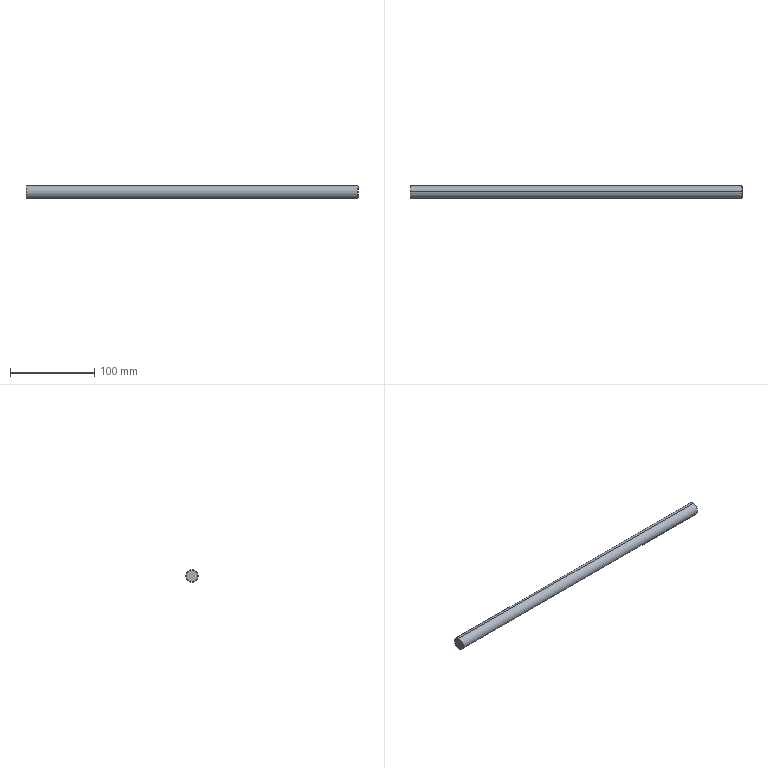Part | STEP file | 0232_005_PSSFG15-395 | 1 solid | 8 faces | box 395 x 15 x 15 mm | volume 69791 mm3 | cone 4 | cylinder 2 | plane 2 | commonest cylinder face diameters 15 x2
STEP:
#1=CARTESIAN_POINT('',(0.,0.,0.));
#2=DIRECTION('',(0.,0.,1.));
#3=DIRECTION('',(1.,0.,0.));
#4=AXIS2_PLACEMENT_3D('',#1,#2,#3);
#5=CARTESIAN_POINT('',(0.5,0.,-7.5));
#6=VERTEX_POINT('',#5);
#7=CARTESIAN_POINT('',(0.5,0.,7.5));
#8=VERTEX_POINT('',#7);
#9=CARTESIAN_POINT('',(0.5,0.,0.));
#10=DIRECTION('',(1.,0.,0.));
#11=DIRECTION('',(0.,0.,-1.));
#12=AXIS2_PLACEMENT_3D('',#9,#10,#11);
#13=CIRCLE('',#12,7.5);
#14=CARTESIAN_POINT('',(197.5,0.,0.));
#15=DIRECTION('',(1.,0.,0.));
#16=DIRECTION('',(0.,0.,-1.));
#17=AXIS2_PLACEMENT_3D('',#14,#15,#16);
#18=CYLINDRICAL_SURFACE('',#17,7.5);
#19=CARTESIAN_POINT('',(0.,-197.));
#20=DIRECTION('',(1.,0.));
#21=VECTOR('',#20,1.);
#22=LINE('',#19,#21);
#23=(GEOMETRIC_REPRESENTATION_CONTEXT(2)PARAMETRIC_REPRESENTATION_CONTEXT()REPRESENTATION_CONTEXT('',''));
#24=DEFINITIONAL_REPRESENTATION('',(#22),#23);
#25=PCURVE('',#18,#24);
#26=CARTESIAN_POINT('',(0.5,0.,0.));
#27=DIRECTION('',(1.,0.,0.));
#28=DIRECTION('',(0.,0.,-1.));
#29=AXIS2_PLACEMENT_3D('',#26,#27,#28);
#30=CONICAL_SURFACE('',#29,7.5,0.7854);
#31=CARTESIAN_POINT('',(0.,0.));
#32=DIRECTION('',(1.,0.));
#33=VECTOR('',#32,1.);
#34=LINE('',#31,#33);
#35=(GEOMETRIC_REPRESENTATION_CONTEXT(2)PARAMETRIC_REPRESENTATION_CONTEXT()REPRESENTATION_CONTEXT('',''));
#36=DEFINITIONAL_REPRESENTATION('',(#34),#35);
#37=PCURVE('',#30,#36);
#38=SURFACE_CURVE('',#13,(#25,#37),.PCURVE_S1.);
#39=EDGE_CURVE('',#6,#8,#38,.T.);
#40=ORIENTED_EDGE('',*,*,#39,.T.);
#41=CARTESIAN_POINT('',(394.5,0.,7.5));
#42=VERTEX_POINT('',#41);
#43=CARTESIAN_POINT('',(197.5,0.,7.5));
#44=DIRECTION('',(1.,0.,0.));
#45=VECTOR('',#44,1.);
#46=LINE('',#43,#45);
#47=CARTESIAN_POINT('',(3.142,0.));
#48=DIRECTION('',(0.,1.));
#49=VECTOR('',#48,1.);
#50=LINE('',#47,#49);
#51=(GEOMETRIC_REPRESENTATION_CONTEXT(2)PARAMETRIC_REPRESENTATION_CONTEXT()REPRESENTATION_CONTEXT('',''));
#52=DEFINITIONAL_REPRESENTATION('',(#50),#51);
#53=PCURVE('',#18,#52);
#54=CARTESIAN_POINT('',(197.5,0.,0.));
#55=DIRECTION('',(1.,0.,0.));
#56=DIRECTION('',(0.,0.,-1.));
#57=AXIS2_PLACEMENT_3D('',#54,#55,#56);
#58=CYLINDRICAL_SURFACE('',#57,7.5);
#59=CARTESIAN_POINT('',(3.142,0.));
#60=DIRECTION('',(0.,1.));
#61=VECTOR('',#60,1.);
#62=LINE('',#59,#61);
#63=(GEOMETRIC_REPRESENTATION_CONTEXT(2)PARAMETRIC_REPRESENTATION_CONTEXT()REPRESENTATION_CONTEXT('',''));
#64=DEFINITIONAL_REPRESENTATION('',(#62),#63);
#65=PCURVE('',#58,#64);
#66=SURFACE_CURVE('',#46,(#53,#65),.PCURVE_S1.);
#67=EDGE_CURVE('',#8,#42,#66,.T.);
#68=ORIENTED_EDGE('',*,*,#67,.T.);
#69=CARTESIAN_POINT('',(394.5,0.,-7.5));
#70=VERTEX_POINT('',#69);
#71=CARTESIAN_POINT('',(394.5,0.,0.));
#72=DIRECTION('',(-1.,0.,0.));
#73=DIRECTION('',(0.,0.,-1.));
#74=AXIS2_PLACEMENT_3D('',#71,#72,#73);
#75=CIRCLE('',#74,7.5);
#76=CARTESIAN_POINT('',(6.283,197.));
#77=DIRECTION('',(-1.,0.));
#78=VECTOR('',#77,1.);
#79=LINE('',#76,#78);
#80=(GEOMETRIC_REPRESENTATION_CONTEXT(2)PARAMETRIC_REPRESENTATION_CONTEXT()REPRESENTATION_CONTEXT('',''));
#81=DEFINITIONAL_REPRESENTATION('',(#79),#80);
#82=PCURVE('',#18,#81);
#83=CARTESIAN_POINT('',(394.5,0.,0.));
#84=DIRECTION('',(-1.,0.,0.));
#85=DIRECTION('',(0.,0.,1.));
#86=AXIS2_PLACEMENT_3D('',#83,#84,#85);
#87=CONICAL_SURFACE('',#86,7.5,0.7854);
#88=CARTESIAN_POINT('',(-3.142,0.));
#89=DIRECTION('',(1.,0.));
#90=VECTOR('',#89,1.);
#91=LINE('',#88,#90);
#92=(GEOMETRIC_REPRESENTATION_CONTEXT(2)PARAMETRIC_REPRESENTATION_CONTEXT()REPRESENTATION_CONTEXT('',''));
#93=DEFINITIONAL_REPRESENTATION('',(#91),#92);
#94=PCURVE('',#87,#93);
#95=SURFACE_CURVE('',#75,(#82,#94),.PCURVE_S1.);
#96=EDGE_CURVE('',#42,#70,#95,.T.);
#97=ORIENTED_EDGE('',*,*,#96,.T.);
#98=CARTESIAN_POINT('',(197.5,0.,-7.5));
#99=DIRECTION('',(1.,0.,0.));
#100=VECTOR('',#99,1.);
#101=LINE('',#98,#100);
#102=CARTESIAN_POINT('',(0.,0.));
#103=DIRECTION('',(0.,1.));
#104=VECTOR('',#103,1.);
#105=LINE('',#102,#104);
#106=(GEOMETRIC_REPRESENTATION_CONTEXT(2)PARAMETRIC_REPRESENTATION_CONTEXT()REPRESENTATION_CONTEXT('',''));
#107=DEFINITIONAL_REPRESENTATION('',(#105),#106);
#108=PCURVE('',#18,#107);
#109=CARTESIAN_POINT('',(6.283,0.));
#110=DIRECTION('',(0.,1.));
#111=VECTOR('',#110,1.);
#112=LINE('',#109,#111);
#113=(GEOMETRIC_REPRESENTATION_CONTEXT(2)PARAMETRIC_REPRESENTATION_CONTEXT()REPRESENTATION_CONTEXT('',''));
#114=DEFINITIONAL_REPRESENTATION('',(#112),#113);
#115=PCURVE('',#58,#114);
#116=SURFACE_CURVE('',#101,(#108,#115),.PCURVE_S1.);
#117=EDGE_CURVE('',#6,#70,#116,.T.);
#118=ORIENTED_EDGE('',*,*,#117,.F.);
#119=EDGE_LOOP('',(#40,#68,#97,#118));
#120=FACE_BOUND('',#119,.T.);
#121=ADVANCED_FACE('',(#120),#18,.T.);
#122=CARTESIAN_POINT('',(0.,0.,-7.));
#123=VERTEX_POINT('',#122);
#124=CARTESIAN_POINT('',(0.,0.,7.));
#125=VERTEX_POINT('',#124);
#126=CARTESIAN_POINT('',(0.,0.,0.));
#127=DIRECTION('',(1.,0.,0.));
#128=DIRECTION('',(0.,0.,-1.));
#129=AXIS2_PLACEMENT_3D('',#126,#127,#128);
#130=CIRCLE('',#129,7.);
#131=CARTESIAN_POINT('',(0.,-0.5));
#132=DIRECTION('',(1.,0.));
#133=VECTOR('',#132,1.);
#134=LINE('',#131,#133);
#135=(GEOMETRIC_REPRESENTATION_CONTEXT(2)PARAMETRIC_REPRESENTATION_CONTEXT()REPRESENTATION_CONTEXT('',''));
#136=DEFINITIONAL_REPRESENTATION('',(#134),#135);
#137=PCURVE('',#30,#136);
#138=CARTESIAN_POINT('',(0.,3.5,0.));
#139=DIRECTION('',(-1.,0.,0.));
#140=DIRECTION('',(0.,0.,1.));
#141=AXIS2_PLACEMENT_3D('',#138,#139,#140);
#142=PLANE('',#141);
#143=CARTESIAN_POINT('',(-7.,-3.5));
#144=CARTESIAN_POINT('',(-7.,8.624));
#145=CARTESIAN_POINT('',(3.5,2.562));
#146=CARTESIAN_POINT('',(14.,-3.5));
#147=CARTESIAN_POINT('',(3.5,-9.562));
#148=CARTESIAN_POINT('',(-7.,-15.624));
#149=CARTESIAN_POINT('',(-7.,-3.5));
#150=(BOUNDED_CURVE()B_SPLINE_CURVE(2,(#143,#144,#145,#146,#147,#148,#149),.UNSPECIFIED.,.T.,.F.)B_SPLINE_CURVE_WITH_KNOTS((1,2,2,2,2,1),(-2.094,0.,2.094,4.189,6.283,8.378),.UNSPECIFIED.)CURVE()GEOMETRIC_REPRESENTATION_ITEM()RATIONAL_B_SPLINE_CURVE((1.,0.5,1.,0.5,1.,0.5,1.))REPRESENTATION_ITEM(''));
#151=(GEOMETRIC_REPRESENTATION_CONTEXT(2)PARAMETRIC_REPRESENTATION_CONTEXT()REPRESENTATION_CONTEXT('',''));
#152=DEFINITIONAL_REPRESENTATION('',(#150),#151);
#153=PCURVE('',#142,#152);
#154=SURFACE_CURVE('',#130,(#137,#153),.PCURVE_S1.);
#155=EDGE_CURVE('',#123,#125,#154,.T.);
#156=ORIENTED_EDGE('',*,*,#155,.T.);
#157=CARTESIAN_POINT('',(0.5,0.,7.5));
#158=DIRECTION('',(0.7071,0.,0.7071));
#159=VECTOR('',#158,1.);
#160=LINE('',#157,#159);
#161=CARTESIAN_POINT('',(3.142,0.));
#162=DIRECTION('',(0.,1.));
#163=VECTOR('',#162,1.);
#164=LINE('',#161,#163);
#165=(GEOMETRIC_REPRESENTATION_CONTEXT(2)PARAMETRIC_REPRESENTATION_CONTEXT()REPRESENTATION_CONTEXT('',''));
#166=DEFINITIONAL_REPRESENTATION('',(#164),#165);
#167=PCURVE('',#30,#166);
#168=CARTESIAN_POINT('',(0.5,0.,0.));
#169=DIRECTION('',(1.,0.,0.));
#170=DIRECTION('',(0.,0.,-1.));
#171=AXIS2_PLACEMENT_3D('',#168,#169,#170);
#172=CONICAL_SURFACE('',#171,7.5,0.7854);
#173=CARTESIAN_POINT('',(3.142,0.));
#174=DIRECTION('',(0.,1.));
#175=VECTOR('',#174,1.);
#176=LINE('',#173,#175);
#177=(GEOMETRIC_REPRESENTATION_CONTEXT(2)PARAMETRIC_REPRESENTATION_CONTEXT()REPRESENTATION_CONTEXT('',''));
#178=DEFINITIONAL_REPRESENTATION('',(#176),#177);
#179=PCURVE('',#172,#178);
#180=SURFACE_CURVE('',#160,(#167,#179),.PCURVE_S1.);
#181=EDGE_CURVE('',#125,#8,#180,.T.);
#182=ORIENTED_EDGE('',*,*,#181,.T.);
#183=ORIENTED_EDGE('',*,*,#39,.F.);
#184=CARTESIAN_POINT('',(0.5,0.,-7.5));
#185=DIRECTION('',(0.7071,0.,-0.7071));
#186=VECTOR('',#185,1.);
#187=LINE('',#184,#186);
#188=CARTESIAN_POINT('',(0.,0.));
#189=DIRECTION('',(0.,1.));
#190=VECTOR('',#189,1.);
#191=LINE('',#188,#190);
#192=(GEOMETRIC_REPRESENTATION_CONTEXT(2)PARAMETRIC_REPRESENTATION_CONTEXT()REPRESENTATION_CONTEXT('',''));
#193=DEFINITIONAL_REPRESENTATION('',(#191),#192);
#194=PCURVE('',#30,#193);
#195=CARTESIAN_POINT('',(6.283,0.));
#196=DIRECTION('',(0.,1.));
#197=VECTOR('',#196,1.);
#198=LINE('',#195,#197);
#199=(GEOMETRIC_REPRESENTATION_CONTEXT(2)PARAMETRIC_REPRESENTATION_CONTEXT()REPRESENTATION_CONTEXT('',''));
#200=DEFINITIONAL_REPRESENTATION('',(#198),#199);
#201=PCURVE('',#172,#200);
#202=SURFACE_CURVE('',#187,(#194,#201),.PCURVE_S1.);
#203=EDGE_CURVE('',#123,#6,#202,.T.);
#204=ORIENTED_EDGE('',*,*,#203,.F.);
#205=EDGE_LOOP('',(#156,#182,#183,#204));
#206=FACE_BOUND('',#205,.T.);
#207=ADVANCED_FACE('',(#206),#30,.T.);
#208=CARTESIAN_POINT('',(395.,0.,7.));
#209=VERTEX_POINT('',#208);
#210=CARTESIAN_POINT('',(395.,0.,-7.));
#211=VERTEX_POINT('',#210);
#212=CARTESIAN_POINT('',(395.,0.,0.));
#213=DIRECTION('',(-1.,0.,0.));
#214=DIRECTION('',(0.,0.,1.));
#215=AXIS2_PLACEMENT_3D('',#212,#213,#214);
#216=CIRCLE('',#215,7.);
#217=CARTESIAN_POINT('',(0.,-0.5));
#218=DIRECTION('',(1.,0.));
#219=VECTOR('',#218,1.);
#220=LINE('',#217,#219);
#221=(GEOMETRIC_REPRESENTATION_CONTEXT(2)PARAMETRIC_REPRESENTATION_CONTEXT()REPRESENTATION_CONTEXT('',''));
#222=DEFINITIONAL_REPRESENTATION('',(#220),#221);
#223=PCURVE('',#87,#222);
#224=CARTESIAN_POINT('',(395.,3.5,0.));
#225=DIRECTION('',(1.,0.,0.));
#226=DIRECTION('',(0.,0.,-1.));
#227=AXIS2_PLACEMENT_3D('',#224,#225,#226);
#228=PLANE('',#227);
#229=CARTESIAN_POINT('',(-7.,-3.5));
#230=CARTESIAN_POINT('',(-7.,8.624));
#231=CARTESIAN_POINT('',(3.5,2.562));
#232=CARTESIAN_POINT('',(14.,-3.5));
#233=CARTESIAN_POINT('',(3.5,-9.562));
#234=CARTESIAN_POINT('',(-7.,-15.624));
#235=CARTESIAN_POINT('',(-7.,-3.5));
#236=(BOUNDED_CURVE()B_SPLINE_CURVE(2,(#229,#230,#231,#232,#233,#234,#235),.UNSPECIFIED.,.T.,.F.)B_SPLINE_CURVE_WITH_KNOTS((1,2,2,2,2,1),(-2.094,0.,2.094,4.189,6.283,8.378),.UNSPECIFIED.)CURVE()GEOMETRIC_REPRESENTATION_ITEM()RATIONAL_B_SPLINE_CURVE((1.,0.5,1.,0.5,1.,0.5,1.))REPRESENTATION_ITEM(''));
#237=(GEOMETRIC_REPRESENTATION_CONTEXT(2)PARAMETRIC_REPRESENTATION_CONTEXT()REPRESENTATION_CONTEXT('',''));
#238=DEFINITIONAL_REPRESENTATION('',(#236),#237);
#239=PCURVE('',#228,#238);
#240=SURFACE_CURVE('',#216,(#223,#239),.PCURVE_S1.);
#241=EDGE_CURVE('',#209,#211,#240,.T.);
#242=ORIENTED_EDGE('',*,*,#241,.T.);
#243=CARTESIAN_POINT('',(394.5,0.,-7.5));
#244=DIRECTION('',(-0.7071,0.,-0.7071));
#245=VECTOR('',#244,1.);
#246=LINE('',#243,#245);
#247=CARTESIAN_POINT('',(3.142,0.));
#248=DIRECTION('',(0.,1.));
#249=VECTOR('',#248,1.);
#250=LINE('',#247,#249);
#251=(GEOMETRIC_REPRESENTATION_CONTEXT(2)PARAMETRIC_REPRESENTATION_CONTEXT()REPRESENTATION_CONTEXT('',''));
#252=DEFINITIONAL_REPRESENTATION('',(#250),#251);
#253=PCURVE('',#87,#252);
#254=CARTESIAN_POINT('',(394.5,0.,0.));
#255=DIRECTION('',(-1.,0.,0.));
#256=DIRECTION('',(0.,0.,1.));
#257=AXIS2_PLACEMENT_3D('',#254,#255,#256);
#258=CONICAL_SURFACE('',#257,7.5,0.7854);
#259=CARTESIAN_POINT('',(3.142,0.));
#260=DIRECTION('',(0.,1.));
#261=VECTOR('',#260,1.);
#262=LINE('',#259,#261);
#263=(GEOMETRIC_REPRESENTATION_CONTEXT(2)PARAMETRIC_REPRESENTATION_CONTEXT()REPRESENTATION_CONTEXT('',''));
#264=DEFINITIONAL_REPRESENTATION('',(#262),#263);
#265=PCURVE('',#258,#264);
#266=SURFACE_CURVE('',#246,(#253,#265),.PCURVE_S1.);
#267=EDGE_CURVE('',#211,#70,#266,.T.);
#268=ORIENTED_EDGE('',*,*,#267,.T.);
#269=ORIENTED_EDGE('',*,*,#96,.F.);
#270=CARTESIAN_POINT('',(394.5,0.,7.5));
#271=DIRECTION('',(-0.7071,0.,0.7071));
#272=VECTOR('',#271,1.);
#273=LINE('',#270,#272);
#274=CARTESIAN_POINT('',(0.,0.));
#275=DIRECTION('',(0.,1.));
#276=VECTOR('',#275,1.);
#277=LINE('',#274,#276);
#278=(GEOMETRIC_REPRESENTATION_CONTEXT(2)PARAMETRIC_REPRESENTATION_CONTEXT()REPRESENTATION_CONTEXT('',''));
#279=DEFINITIONAL_REPRESENTATION('',(#277),#278);
#280=PCURVE('',#87,#279);
#281=CARTESIAN_POINT('',(6.283,0.));
#282=DIRECTION('',(0.,1.));
#283=VECTOR('',#282,1.);
#284=LINE('',#281,#283);
#285=(GEOMETRIC_REPRESENTATION_CONTEXT(2)PARAMETRIC_REPRESENTATION_CONTEXT()REPRESENTATION_CONTEXT('',''));
#286=DEFINITIONAL_REPRESENTATION('',(#284),#285);
#287=PCURVE('',#258,#286);
#288=SURFACE_CURVE('',#273,(#280,#287),.PCURVE_S1.);
#289=EDGE_CURVE('',#209,#42,#288,.T.);
#290=ORIENTED_EDGE('',*,*,#289,.F.);
#291=EDGE_LOOP('',(#242,#268,#269,#290));
#292=FACE_BOUND('',#291,.T.);
#293=ADVANCED_FACE('',(#292),#87,.T.);
#294=ORIENTED_EDGE('',*,*,#67,.F.);
#295=CARTESIAN_POINT('',(0.5,0.,0.));
#296=DIRECTION('',(1.,0.,0.));
#297=DIRECTION('',(0.,0.,-1.));
#298=AXIS2_PLACEMENT_3D('',#295,#296,#297);
#299=CIRCLE('',#298,7.5);
#300=CARTESIAN_POINT('',(0.,-197.));
#301=DIRECTION('',(1.,0.));
#302=VECTOR('',#301,1.);
#303=LINE('',#300,#302);
#304=(GEOMETRIC_REPRESENTATION_CONTEXT(2)PARAMETRIC_REPRESENTATION_CONTEXT()REPRESENTATION_CONTEXT('',''));
#305=DEFINITIONAL_REPRESENTATION('',(#303),#304);
#306=PCURVE('',#58,#305);
#307=CARTESIAN_POINT('',(0.,0.));
#308=DIRECTION('',(1.,0.));
#309=VECTOR('',#308,1.);
#310=LINE('',#307,#309);
#311=(GEOMETRIC_REPRESENTATION_CONTEXT(2)PARAMETRIC_REPRESENTATION_CONTEXT()REPRESENTATION_CONTEXT('',''));
#312=DEFINITIONAL_REPRESENTATION('',(#310),#311);
#313=PCURVE('',#172,#312);
#314=SURFACE_CURVE('',#299,(#306,#313),.PCURVE_S1.);
#315=EDGE_CURVE('',#8,#6,#314,.T.);
#316=ORIENTED_EDGE('',*,*,#315,.T.);
#317=ORIENTED_EDGE('',*,*,#117,.T.);
#318=CARTESIAN_POINT('',(394.5,0.,0.));
#319=DIRECTION('',(-1.,0.,0.));
#320=DIRECTION('',(0.,0.,-1.));
#321=AXIS2_PLACEMENT_3D('',#318,#319,#320);
#322=CIRCLE('',#321,7.5);
#323=CARTESIAN_POINT('',(6.283,197.));
#324=DIRECTION('',(-1.,0.));
#325=VECTOR('',#324,1.);
#326=LINE('',#323,#325);
#327=(GEOMETRIC_REPRESENTATION_CONTEXT(2)PARAMETRIC_REPRESENTATION_CONTEXT()REPRESENTATION_CONTEXT('',''));
#328=DEFINITIONAL_REPRESENTATION('',(#326),#327);
#329=PCURVE('',#58,#328);
#330=CARTESIAN_POINT('',(3.142,0.));
#331=DIRECTION('',(1.,0.));
#332=VECTOR('',#331,1.);
#333=LINE('',#330,#332);
#334=(GEOMETRIC_REPRESENTATION_CONTEXT(2)PARAMETRIC_REPRESENTATION_CONTEXT()REPRESENTATION_CONTEXT('',''));
#335=DEFINITIONAL_REPRESENTATION('',(#333),#334);
#336=PCURVE('',#258,#335);
#337=SURFACE_CURVE('',#322,(#329,#336),.PCURVE_S1.);
#338=EDGE_CURVE('',#70,#42,#337,.T.);
#339=ORIENTED_EDGE('',*,*,#338,.T.);
#340=EDGE_LOOP('',(#294,#316,#317,#339));
#341=FACE_BOUND('',#340,.T.);
#342=ADVANCED_FACE('',(#341),#58,.T.);
#343=ORIENTED_EDGE('',*,*,#181,.F.);
#344=CARTESIAN_POINT('',(0.,0.,0.));
#345=DIRECTION('',(1.,0.,0.));
#346=DIRECTION('',(0.,0.,-1.));
#347=AXIS2_PLACEMENT_3D('',#344,#345,#346);
#348=CIRCLE('',#347,7.);
#349=CARTESIAN_POINT('',(0.,-0.5));
#350=DIRECTION('',(1.,0.));
#351=VECTOR('',#350,1.);
#352=LINE('',#349,#351);
#353=(GEOMETRIC_REPRESENTATION_CONTEXT(2)PARAMETRIC_REPRESENTATION_CONTEXT()REPRESENTATION_CONTEXT('',''));
#354=DEFINITIONAL_REPRESENTATION('',(#352),#353);
#355=PCURVE('',#172,#354);
#356=CARTESIAN_POINT('',(-7.,-3.5));
#357=CARTESIAN_POINT('',(-7.,8.624));
#358=CARTESIAN_POINT('',(3.5,2.562));
#359=CARTESIAN_POINT('',(14.,-3.5));
#360=CARTESIAN_POINT('',(3.5,-9.562));
#361=CARTESIAN_POINT('',(-7.,-15.624));
#362=CARTESIAN_POINT('',(-7.,-3.5));
#363=(BOUNDED_CURVE()B_SPLINE_CURVE(2,(#356,#357,#358,#359,#360,#361,#362),.UNSPECIFIED.,.T.,.F.)B_SPLINE_CURVE_WITH_KNOTS((1,2,2,2,2,1),(-2.094,0.,2.094,4.189,6.283,8.378),.UNSPECIFIED.)CURVE()GEOMETRIC_REPRESENTATION_ITEM()RATIONAL_B_SPLINE_CURVE((1.,0.5,1.,0.5,1.,0.5,1.))REPRESENTATION_ITEM(''));
#364=(GEOMETRIC_REPRESENTATION_CONTEXT(2)PARAMETRIC_REPRESENTATION_CONTEXT()REPRESENTATION_CONTEXT('',''));
#365=DEFINITIONAL_REPRESENTATION('',(#363),#364);
#366=PCURVE('',#142,#365);
#367=SURFACE_CURVE('',#348,(#355,#366),.PCURVE_S1.);
#368=EDGE_CURVE('',#125,#123,#367,.T.);
#369=ORIENTED_EDGE('',*,*,#368,.T.);
#370=ORIENTED_EDGE('',*,*,#203,.T.);
#371=ORIENTED_EDGE('',*,*,#315,.F.);
#372=EDGE_LOOP('',(#343,#369,#370,#371));
#373=FACE_BOUND('',#372,.T.);
#374=ADVANCED_FACE('',(#373),#172,.T.);
#375=ORIENTED_EDGE('',*,*,#267,.F.);
#376=CARTESIAN_POINT('',(395.,0.,0.));
#377=DIRECTION('',(-1.,0.,0.));
#378=DIRECTION('',(0.,0.,1.));
#379=AXIS2_PLACEMENT_3D('',#376,#377,#378);
#380=CIRCLE('',#379,7.);
#381=CARTESIAN_POINT('',(0.,-0.5));
#382=DIRECTION('',(1.,0.));
#383=VECTOR('',#382,1.);
#384=LINE('',#381,#383);
#385=(GEOMETRIC_REPRESENTATION_CONTEXT(2)PARAMETRIC_REPRESENTATION_CONTEXT()REPRESENTATION_CONTEXT('',''));
#386=DEFINITIONAL_REPRESENTATION('',(#384),#385);
#387=PCURVE('',#258,#386);
#388=CARTESIAN_POINT('',(-7.,-3.5));
#389=CARTESIAN_POINT('',(-7.,8.624));
#390=CARTESIAN_POINT('',(3.5,2.562));
#391=CARTESIAN_POINT('',(14.,-3.5));
#392=CARTESIAN_POINT('',(3.5,-9.562));
#393=CARTESIAN_POINT('',(-7.,-15.624));
#394=CARTESIAN_POINT('',(-7.,-3.5));
#395=(BOUNDED_CURVE()B_SPLINE_CURVE(2,(#388,#389,#390,#391,#392,#393,#394),.UNSPECIFIED.,.T.,.F.)B_SPLINE_CURVE_WITH_KNOTS((1,2,2,2,2,1),(-2.094,0.,2.094,4.189,6.283,8.378),.UNSPECIFIED.)CURVE()GEOMETRIC_REPRESENTATION_ITEM()RATIONAL_B_SPLINE_CURVE((1.,0.5,1.,0.5,1.,0.5,1.))REPRESENTATION_ITEM(''));
#396=(GEOMETRIC_REPRESENTATION_CONTEXT(2)PARAMETRIC_REPRESENTATION_CONTEXT()REPRESENTATION_CONTEXT('',''));
#397=DEFINITIONAL_REPRESENTATION('',(#395),#396);
#398=PCURVE('',#228,#397);
#399=SURFACE_CURVE('',#380,(#387,#398),.PCURVE_S1.);
#400=EDGE_CURVE('',#211,#209,#399,.T.);
#401=ORIENTED_EDGE('',*,*,#400,.T.);
#402=ORIENTED_EDGE('',*,*,#289,.T.);
#403=ORIENTED_EDGE('',*,*,#338,.F.);
#404=EDGE_LOOP('',(#375,#401,#402,#403));
#405=FACE_BOUND('',#404,.T.);
#406=ADVANCED_FACE('',(#405),#258,.T.);
#407=ORIENTED_EDGE('',*,*,#155,.F.);
#408=ORIENTED_EDGE('',*,*,#368,.F.);
#409=EDGE_LOOP('',(#407,#408));
#410=FACE_BOUND('',#409,.T.);
#411=ADVANCED_FACE('',(#410),#142,.T.);
#412=ORIENTED_EDGE('',*,*,#241,.F.);
#413=ORIENTED_EDGE('',*,*,#400,.F.);
#414=EDGE_LOOP('',(#412,#413));
#415=FACE_BOUND('',#414,.T.);
#416=ADVANCED_FACE('',(#415),#228,.T.);
#417=CLOSED_SHELL('',(#121,#207,#293,#342,#374,#406,#411,#416));
#418=MANIFOLD_SOLID_BREP('',#417);
#419=(LENGTH_UNIT()NAMED_UNIT(*)SI_UNIT(.MILLI.,.METRE.));
#420=UNCERTAINTY_MEASURE_WITH_UNIT(LENGTH_MEASURE(0.0000001),#419,'','');
#421=(NAMED_UNIT(*)PLANE_ANGLE_UNIT()SI_UNIT($,.RADIAN.));
#422=(NAMED_UNIT(*)SI_UNIT($,.STERADIAN.)SOLID_ANGLE_UNIT());
#423=(GEOMETRIC_REPRESENTATION_CONTEXT(3)GLOBAL_UNCERTAINTY_ASSIGNED_CONTEXT((#420))GLOBAL_UNIT_ASSIGNED_CONTEXT((#419,#421,#422))REPRESENTATION_CONTEXT('',''));
#424=ADVANCED_BREP_SHAPE_REPRESENTATION('',(#4,#418),#423);